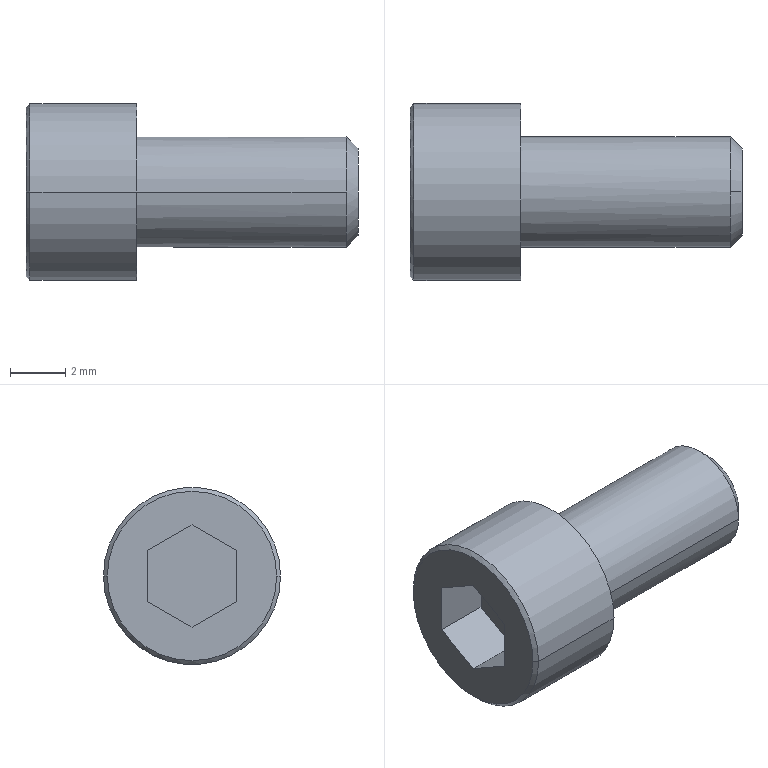Part | NX | features BREP 1 | 1 solid | 18 faces | box 12 x 6.4 x 6.4 mm | volume 210.2 mm3 | plane 10 | cylinder 4 | cone 4 | commonest cylinder face diameters 4 x2 6.4 x2
STEP:
#1=CARTESIAN_POINT('',(4.,2.,0.));
#2=VERTEX_POINT('',#1);
#3=CARTESIAN_POINT('',(4.,-2.,0.));
#4=VERTEX_POINT('',#3);
#5=CARTESIAN_POINT('',(4.,0.,0.));
#6=DIRECTION('',(1.,0.,0.));
#7=DIRECTION('',(0.,1.,0.));
#8=AXIS2_PLACEMENT_3D('',#5,#6,#7);
#9=CIRCLE('',#8,2.);
#10=EDGE_CURVE('',#2,#4,#9,.T.);
#11=ORIENTED_EDGE('',*,*,#10,.T.);
#12=CARTESIAN_POINT('',(11.57,-2.,0.));
#13=VERTEX_POINT('',#12);
#14=CARTESIAN_POINT('',(0.,-2.,0.));
#15=DIRECTION('',(1.,0.,0.));
#16=VECTOR('',#15,1000.);
#17=LINE('',#14,#16);
#18=EDGE_CURVE('',#4,#13,#17,.T.);
#19=ORIENTED_EDGE('',*,*,#18,.T.);
#20=CARTESIAN_POINT('',(11.57,0.,2.));
#21=VERTEX_POINT('',#20);
#22=CARTESIAN_POINT('',(11.57,0.,0.));
#23=DIRECTION('',(-1.,0.,0.));
#24=DIRECTION('',(0.,1.,0.));
#25=AXIS2_PLACEMENT_3D('',#22,#23,#24);
#26=CIRCLE('',#25,2.);
#27=EDGE_CURVE('',#13,#21,#26,.T.);
#28=ORIENTED_EDGE('',*,*,#27,.T.);
#29=CARTESIAN_POINT('',(11.57,2.,0.));
#30=VERTEX_POINT('',#29);
#31=CARTESIAN_POINT('',(11.57,0.,0.));
#32=DIRECTION('',(-1.,0.,0.));
#33=DIRECTION('',(0.,1.,0.));
#34=AXIS2_PLACEMENT_3D('',#31,#32,#33);
#35=CIRCLE('',#34,2.);
#36=EDGE_CURVE('',#21,#30,#35,.T.);
#37=ORIENTED_EDGE('',*,*,#36,.T.);
#38=CARTESIAN_POINT('',(0.,2.,0.));
#39=DIRECTION('',(1.,0.,0.));
#40=VECTOR('',#39,1000.);
#41=LINE('',#38,#40);
#42=EDGE_CURVE('',#2,#30,#41,.T.);
#43=ORIENTED_EDGE('',*,*,#42,.F.);
#44=EDGE_LOOP('',(#11,#19,#28,#37,#43));
#45=FACE_BOUND('',#44,.T.);
#46=CARTESIAN_POINT('',(0.,0.,0.));
#47=DIRECTION('',(1.,0.,0.));
#48=DIRECTION('',(0.,-1.,0.));
#49=AXIS2_PLACEMENT_3D('',#46,#47,#48);
#50=CYLINDRICAL_SURFACE('',#49,2.);
#51=ADVANCED_FACE('',(#45),#50,.T.);
#52=CARTESIAN_POINT('',(12.,0.,1.571));
#53=VERTEX_POINT('',#52);
#54=CARTESIAN_POINT('',(12.,0.,-1.571));
#55=VERTEX_POINT('',#54);
#56=CARTESIAN_POINT('',(12.,0.,0.));
#57=DIRECTION('',(-1.,0.,0.));
#58=DIRECTION('',(0.,0.,1.));
#59=AXIS2_PLACEMENT_3D('',#56,#57,#58);
#60=CIRCLE('',#59,1.571);
#61=EDGE_CURVE('',#53,#55,#60,.T.);
#62=ORIENTED_EDGE('',*,*,#61,.T.);
#63=CARTESIAN_POINT('',(11.57,0.,-2.));
#64=VERTEX_POINT('',#63);
#65=CARTESIAN_POINT('',(11.571,0.,-2.));
#66=DIRECTION('',(-0.7071,0.,-0.7071));
#67=VECTOR('',#66,1000.);
#68=LINE('',#65,#67);
#69=EDGE_CURVE('',#55,#64,#68,.T.);
#70=ORIENTED_EDGE('',*,*,#69,.T.);
#71=CARTESIAN_POINT('',(11.57,0.,0.));
#72=DIRECTION('',(-1.,0.,0.));
#73=DIRECTION('',(0.,1.,0.));
#74=AXIS2_PLACEMENT_3D('',#71,#72,#73);
#75=CIRCLE('',#74,2.);
#76=EDGE_CURVE('',#30,#64,#75,.T.);
#77=ORIENTED_EDGE('',*,*,#76,.F.);
#78=ORIENTED_EDGE('',*,*,#36,.F.);
#79=CARTESIAN_POINT('',(11.571,0.,2.));
#80=DIRECTION('',(-0.7071,0.,0.7071));
#81=VECTOR('',#80,1000.);
#82=LINE('',#79,#81);
#83=EDGE_CURVE('',#53,#21,#82,.T.);
#84=ORIENTED_EDGE('',*,*,#83,.F.);
#85=EDGE_LOOP('',(#62,#70,#77,#78,#84));
#86=FACE_BOUND('',#85,.T.);
#87=CARTESIAN_POINT('',(11.571,0.,0.));
#88=DIRECTION('',(-1.,0.,0.));
#89=DIRECTION('',(0.,0.,-1.));
#90=AXIS2_PLACEMENT_3D('',#87,#88,#89);
#91=CONICAL_SURFACE('',#90,2.,0.7854);
#92=ADVANCED_FACE('',(#86),#91,.T.);
#93=CARTESIAN_POINT('',(0.1414,3.2,0.));
#94=VERTEX_POINT('',#93);
#95=CARTESIAN_POINT('',(0.1414,-3.2,0.));
#96=VERTEX_POINT('',#95);
#97=CARTESIAN_POINT('',(0.1414,0.,0.));
#98=DIRECTION('',(1.,0.,0.));
#99=DIRECTION('',(0.,1.,0.));
#100=AXIS2_PLACEMENT_3D('',#97,#98,#99);
#101=CIRCLE('',#100,3.2);
#102=EDGE_CURVE('',#94,#96,#101,.T.);
#103=ORIENTED_EDGE('',*,*,#102,.T.);
#104=CARTESIAN_POINT('',(4.,-3.2,0.));
#105=VERTEX_POINT('',#104);
#106=CARTESIAN_POINT('',(0.,-3.2,0.));
#107=DIRECTION('',(1.,0.,0.));
#108=VECTOR('',#107,1000.);
#109=LINE('',#106,#108);
#110=EDGE_CURVE('',#96,#105,#109,.T.);
#111=ORIENTED_EDGE('',*,*,#110,.T.);
#112=CARTESIAN_POINT('',(4.,3.2,0.));
#113=VERTEX_POINT('',#112);
#114=CARTESIAN_POINT('',(4.,0.,0.));
#115=DIRECTION('',(-1.,0.,0.));
#116=DIRECTION('',(0.,1.,0.));
#117=AXIS2_PLACEMENT_3D('',#114,#115,#116);
#118=CIRCLE('',#117,3.2);
#119=EDGE_CURVE('',#105,#113,#118,.T.);
#120=ORIENTED_EDGE('',*,*,#119,.T.);
#121=CARTESIAN_POINT('',(0.,3.2,0.));
#122=DIRECTION('',(1.,0.,0.));
#123=VECTOR('',#122,1000.);
#124=LINE('',#121,#123);
#125=EDGE_CURVE('',#94,#113,#124,.T.);
#126=ORIENTED_EDGE('',*,*,#125,.F.);
#127=EDGE_LOOP('',(#103,#111,#120,#126));
#128=FACE_BOUND('',#127,.T.);
#129=CARTESIAN_POINT('',(0.,0.,0.));
#130=DIRECTION('',(1.,0.,0.));
#131=DIRECTION('',(0.,-1.,0.));
#132=AXIS2_PLACEMENT_3D('',#129,#130,#131);
#133=CYLINDRICAL_SURFACE('',#132,3.2);
#134=ADVANCED_FACE('',(#128),#133,.T.);
#135=CARTESIAN_POINT('',(0.,3.059,0.));
#136=VERTEX_POINT('',#135);
#137=CARTESIAN_POINT('',(0.,-3.059,0.));
#138=VERTEX_POINT('',#137);
#139=CARTESIAN_POINT('',(0.,0.,0.));
#140=DIRECTION('',(1.,0.,0.));
#141=DIRECTION('',(0.,1.,0.));
#142=AXIS2_PLACEMENT_3D('',#139,#140,#141);
#143=CIRCLE('',#142,3.059);
#144=EDGE_CURVE('',#136,#138,#143,.T.);
#145=ORIENTED_EDGE('',*,*,#144,.T.);
#146=CARTESIAN_POINT('',(0.1414,-3.2,0.));
#147=DIRECTION('',(0.7071,-0.7071,0.));
#148=VECTOR('',#147,1000.);
#149=LINE('',#146,#148);
#150=EDGE_CURVE('',#138,#96,#149,.T.);
#151=ORIENTED_EDGE('',*,*,#150,.T.);
#152=ORIENTED_EDGE('',*,*,#102,.F.);
#153=CARTESIAN_POINT('',(0.1414,3.2,0.));
#154=DIRECTION('',(0.7071,0.7071,0.));
#155=VECTOR('',#154,1000.);
#156=LINE('',#153,#155);
#157=EDGE_CURVE('',#136,#94,#156,.T.);
#158=ORIENTED_EDGE('',*,*,#157,.F.);
#159=EDGE_LOOP('',(#145,#151,#152,#158));
#160=FACE_BOUND('',#159,.T.);
#161=CARTESIAN_POINT('',(0.1414,0.,0.));
#162=DIRECTION('',(1.,0.,0.));
#163=DIRECTION('',(0.,-1.,0.));
#164=AXIS2_PLACEMENT_3D('',#161,#162,#163);
#165=CONICAL_SURFACE('',#164,3.2,0.7854);
#166=ADVANCED_FACE('',(#160),#165,.T.);
#167=ORIENTED_EDGE('',*,*,#18,.F.);
#168=CARTESIAN_POINT('',(4.,0.,0.));
#169=DIRECTION('',(1.,0.,0.));
#170=DIRECTION('',(0.,1.,0.));
#171=AXIS2_PLACEMENT_3D('',#168,#169,#170);
#172=CIRCLE('',#171,2.);
#173=EDGE_CURVE('',#4,#2,#172,.T.);
#174=ORIENTED_EDGE('',*,*,#173,.T.);
#175=ORIENTED_EDGE('',*,*,#42,.T.);
#176=ORIENTED_EDGE('',*,*,#76,.T.);
#177=CARTESIAN_POINT('',(11.57,0.,0.));
#178=DIRECTION('',(-1.,0.,0.));
#179=DIRECTION('',(0.,1.,0.));
#180=AXIS2_PLACEMENT_3D('',#177,#178,#179);
#181=CIRCLE('',#180,2.);
#182=EDGE_CURVE('',#64,#13,#181,.T.);
#183=ORIENTED_EDGE('',*,*,#182,.T.);
#184=EDGE_LOOP('',(#167,#174,#175,#176,#183));
#185=FACE_BOUND('',#184,.T.);
#186=CARTESIAN_POINT('',(0.,0.,0.));
#187=DIRECTION('',(1.,0.,0.));
#188=DIRECTION('',(0.,-1.,0.));
#189=AXIS2_PLACEMENT_3D('',#186,#187,#188);
#190=CYLINDRICAL_SURFACE('',#189,2.);
#191=ADVANCED_FACE('',(#185),#190,.T.);
#192=ORIENTED_EDGE('',*,*,#69,.F.);
#193=CARTESIAN_POINT('',(12.,0.,0.));
#194=DIRECTION('',(-1.,0.,0.));
#195=DIRECTION('',(0.,0.,1.));
#196=AXIS2_PLACEMENT_3D('',#193,#194,#195);
#197=CIRCLE('',#196,1.571);
#198=EDGE_CURVE('',#55,#53,#197,.T.);
#199=ORIENTED_EDGE('',*,*,#198,.T.);
#200=ORIENTED_EDGE('',*,*,#83,.T.);
#201=ORIENTED_EDGE('',*,*,#27,.F.);
#202=ORIENTED_EDGE('',*,*,#182,.F.);
#203=EDGE_LOOP('',(#192,#199,#200,#201,#202));
#204=FACE_BOUND('',#203,.T.);
#205=CARTESIAN_POINT('',(11.571,0.,0.));
#206=DIRECTION('',(-1.,0.,0.));
#207=DIRECTION('',(0.,0.,-1.));
#208=AXIS2_PLACEMENT_3D('',#205,#206,#207);
#209=CONICAL_SURFACE('',#208,2.,0.7854);
#210=ADVANCED_FACE('',(#204),#209,.T.);
#211=ORIENTED_EDGE('',*,*,#10,.F.);
#212=ORIENTED_EDGE('',*,*,#173,.F.);
#213=EDGE_LOOP('',(#211,#212));
#214=FACE_BOUND('',#213,.T.);
#215=CARTESIAN_POINT('',(4.,0.,0.));
#216=DIRECTION('',(-1.,0.,0.));
#217=DIRECTION('',(0.,1.,0.));
#218=AXIS2_PLACEMENT_3D('',#215,#216,#217);
#219=CIRCLE('',#218,3.2);
#220=EDGE_CURVE('',#113,#105,#219,.T.);
#221=ORIENTED_EDGE('',*,*,#220,.F.);
#222=ORIENTED_EDGE('',*,*,#119,.F.);
#223=EDGE_LOOP('',(#221,#222));
#224=FACE_BOUND('',#223,.T.);
#225=CARTESIAN_POINT('',(4.,-2.,0.));
#226=DIRECTION('',(-1.,0.,0.));
#227=DIRECTION('',(0.,1.,0.));
#228=AXIS2_PLACEMENT_3D('',#225,#226,#227);
#229=PLANE('',#228);
#230=ADVANCED_FACE('',(#214,#224),#229,.F.);
#231=ORIENTED_EDGE('',*,*,#61,.F.);
#232=ORIENTED_EDGE('',*,*,#198,.F.);
#233=EDGE_LOOP('',(#231,#232));
#234=FACE_BOUND('',#233,.T.);
#235=CARTESIAN_POINT('',(12.,0.,0.));
#236=DIRECTION('',(-1.,0.,0.));
#237=DIRECTION('',(0.,1.,0.));
#238=AXIS2_PLACEMENT_3D('',#235,#236,#237);
#239=PLANE('',#238);
#240=ADVANCED_FACE('',(#234),#239,.F.);
#241=ORIENTED_EDGE('',*,*,#110,.F.);
#242=CARTESIAN_POINT('',(0.1414,0.,0.));
#243=DIRECTION('',(1.,0.,0.));
#244=DIRECTION('',(0.,1.,0.));
#245=AXIS2_PLACEMENT_3D('',#242,#243,#244);
#246=CIRCLE('',#245,3.2);
#247=EDGE_CURVE('',#96,#94,#246,.T.);
#248=ORIENTED_EDGE('',*,*,#247,.T.);
#249=ORIENTED_EDGE('',*,*,#125,.T.);
#250=ORIENTED_EDGE('',*,*,#220,.T.);
#251=EDGE_LOOP('',(#241,#248,#249,#250));
#252=FACE_BOUND('',#251,.T.);
#253=CARTESIAN_POINT('',(0.,0.,0.));
#254=DIRECTION('',(1.,0.,0.));
#255=DIRECTION('',(0.,-1.,0.));
#256=AXIS2_PLACEMENT_3D('',#253,#254,#255);
#257=CYLINDRICAL_SURFACE('',#256,3.2);
#258=ADVANCED_FACE('',(#252),#257,.T.);
#259=ORIENTED_EDGE('',*,*,#150,.F.);
#260=CARTESIAN_POINT('',(0.,0.,0.));
#261=DIRECTION('',(1.,0.,0.));
#262=DIRECTION('',(0.,1.,0.));
#263=AXIS2_PLACEMENT_3D('',#260,#261,#262);
#264=CIRCLE('',#263,3.059);
#265=EDGE_CURVE('',#138,#136,#264,.T.);
#266=ORIENTED_EDGE('',*,*,#265,.T.);
#267=ORIENTED_EDGE('',*,*,#157,.T.);
#268=ORIENTED_EDGE('',*,*,#247,.F.);
#269=EDGE_LOOP('',(#259,#266,#267,#268));
#270=FACE_BOUND('',#269,.T.);
#271=CARTESIAN_POINT('',(0.1414,0.,0.));
#272=DIRECTION('',(1.,0.,0.));
#273=DIRECTION('',(0.,-1.,0.));
#274=AXIS2_PLACEMENT_3D('',#271,#272,#273);
#275=CONICAL_SURFACE('',#274,3.2,0.7854);
#276=ADVANCED_FACE('',(#270),#275,.T.);
#277=ORIENTED_EDGE('',*,*,#144,.F.);
#278=ORIENTED_EDGE('',*,*,#265,.F.);
#279=EDGE_LOOP('',(#277,#278));
#280=FACE_BOUND('',#279,.T.);
#281=CARTESIAN_POINT('',(0.,0.,-1.848));
#282=VERTEX_POINT('',#281);
#283=CARTESIAN_POINT('',(0.,-1.6,-0.9238));
#284=VERTEX_POINT('',#283);
#285=CARTESIAN_POINT('',(0.,0.,-1.848));
#286=DIRECTION('',(0.,-0.866,0.5));
#287=VECTOR('',#286,1000.);
#288=LINE('',#285,#287);
#289=EDGE_CURVE('',#282,#284,#288,.T.);
#290=ORIENTED_EDGE('',*,*,#289,.F.);
#291=CARTESIAN_POINT('',(0.,1.6,-0.9238));
#292=VERTEX_POINT('',#291);
#293=CARTESIAN_POINT('',(0.,1.6,-0.9238));
#294=DIRECTION('',(0.,-0.866,-0.5));
#295=VECTOR('',#294,1000.);
#296=LINE('',#293,#295);
#297=EDGE_CURVE('',#292,#282,#296,.T.);
#298=ORIENTED_EDGE('',*,*,#297,.F.);
#299=CARTESIAN_POINT('',(0.,1.6,0.9238));
#300=VERTEX_POINT('',#299);
#301=CARTESIAN_POINT('',(0.,1.6,0.));
#302=DIRECTION('',(0.,0.,-1.));
#303=VECTOR('',#302,1000.);
#304=LINE('',#301,#303);
#305=EDGE_CURVE('',#300,#292,#304,.T.);
#306=ORIENTED_EDGE('',*,*,#305,.F.);
#307=CARTESIAN_POINT('',(0.,0.,1.848));
#308=VERTEX_POINT('',#307);
#309=CARTESIAN_POINT('',(0.,0.,1.848));
#310=DIRECTION('',(0.,0.866,-0.5));
#311=VECTOR('',#310,1000.);
#312=LINE('',#309,#311);
#313=EDGE_CURVE('',#308,#300,#312,.T.);
#314=ORIENTED_EDGE('',*,*,#313,.F.);
#315=CARTESIAN_POINT('',(0.,-1.6,0.9238));
#316=VERTEX_POINT('',#315);
#317=CARTESIAN_POINT('',(0.,-1.6,0.9238));
#318=DIRECTION('',(0.,0.866,0.5));
#319=VECTOR('',#318,1000.);
#320=LINE('',#317,#319);
#321=EDGE_CURVE('',#316,#308,#320,.T.);
#322=ORIENTED_EDGE('',*,*,#321,.F.);
#323=CARTESIAN_POINT('',(0.,-1.6,0.));
#324=DIRECTION('',(0.,0.,1.));
#325=VECTOR('',#324,1000.);
#326=LINE('',#323,#325);
#327=EDGE_CURVE('',#284,#316,#326,.T.);
#328=ORIENTED_EDGE('',*,*,#327,.F.);
#329=EDGE_LOOP('',(#290,#298,#306,#314,#322,#328));
#330=FACE_BOUND('',#329,.T.);
#331=CARTESIAN_POINT('',(0.,-3.059,0.));
#332=DIRECTION('',(1.,0.,0.));
#333=DIRECTION('',(0.,-1.,0.));
#334=AXIS2_PLACEMENT_3D('',#331,#332,#333);
#335=PLANE('',#334);
#336=ADVANCED_FACE('',(#280,#330),#335,.F.);
#337=ORIENTED_EDGE('',*,*,#327,.T.);
#338=CARTESIAN_POINT('',(2.,-1.6,0.9238));
#339=VERTEX_POINT('',#338);
#340=CARTESIAN_POINT('',(2.,-1.6,0.9238));
#341=DIRECTION('',(-1.,0.,0.));
#342=VECTOR('',#341,1000.);
#343=LINE('',#340,#342);
#344=EDGE_CURVE('',#339,#316,#343,.T.);
#345=ORIENTED_EDGE('',*,*,#344,.F.);
#346=CARTESIAN_POINT('',(2.,-1.6,-0.9238));
#347=VERTEX_POINT('',#346);
#348=CARTESIAN_POINT('',(2.,-1.6,-0.9238));
#349=DIRECTION('',(0.,0.,1.));
#350=VECTOR('',#349,1000.);
#351=LINE('',#348,#350);
#352=EDGE_CURVE('',#347,#339,#351,.T.);
#353=ORIENTED_EDGE('',*,*,#352,.F.);
#354=CARTESIAN_POINT('',(2.,-1.6,-0.9238));
#355=DIRECTION('',(1.,0.,0.));
#356=VECTOR('',#355,1000.);
#357=LINE('',#354,#356);
#358=EDGE_CURVE('',#284,#347,#357,.T.);
#359=ORIENTED_EDGE('',*,*,#358,.F.);
#360=EDGE_LOOP('',(#337,#345,#353,#359));
#361=FACE_BOUND('',#360,.T.);
#362=CARTESIAN_POINT('',(2.,-1.6,-0.9238));
#363=DIRECTION('',(0.,-1.,0.));
#364=DIRECTION('',(0.,0.,1.));
#365=AXIS2_PLACEMENT_3D('',#362,#363,#364);
#366=PLANE('',#365);
#367=ADVANCED_FACE('',(#361),#366,.F.);
#368=ORIENTED_EDGE('',*,*,#358,.T.);
#369=CARTESIAN_POINT('',(2.,0.,-1.848));
#370=VERTEX_POINT('',#369);
#371=CARTESIAN_POINT('',(2.,0.,-1.848));
#372=DIRECTION('',(0.,-0.866,0.5));
#373=VECTOR('',#372,1000.);
#374=LINE('',#371,#373);
#375=EDGE_CURVE('',#370,#347,#374,.T.);
#376=ORIENTED_EDGE('',*,*,#375,.F.);
#377=CARTESIAN_POINT('',(2.,0.,-1.848));
#378=DIRECTION('',(1.,0.,0.));
#379=VECTOR('',#378,1000.);
#380=LINE('',#377,#379);
#381=EDGE_CURVE('',#282,#370,#380,.T.);
#382=ORIENTED_EDGE('',*,*,#381,.F.);
#383=ORIENTED_EDGE('',*,*,#289,.T.);
#384=EDGE_LOOP('',(#368,#376,#382,#383));
#385=FACE_BOUND('',#384,.T.);
#386=CARTESIAN_POINT('',(2.,0.,-1.848));
#387=DIRECTION('',(0.,-0.5,-0.866));
#388=DIRECTION('',(0.,-0.866,0.5));
#389=AXIS2_PLACEMENT_3D('',#386,#387,#388);
#390=PLANE('',#389);
#391=ADVANCED_FACE('',(#385),#390,.F.);
#392=ORIENTED_EDGE('',*,*,#381,.T.);
#393=CARTESIAN_POINT('',(2.,1.6,-0.9238));
#394=VERTEX_POINT('',#393);
#395=CARTESIAN_POINT('',(2.,1.6,-0.9238));
#396=DIRECTION('',(0.,-0.866,-0.5));
#397=VECTOR('',#396,1000.);
#398=LINE('',#395,#397);
#399=EDGE_CURVE('',#394,#370,#398,.T.);
#400=ORIENTED_EDGE('',*,*,#399,.F.);
#401=CARTESIAN_POINT('',(2.,1.6,-0.9238));
#402=DIRECTION('',(1.,0.,0.));
#403=VECTOR('',#402,1000.);
#404=LINE('',#401,#403);
#405=EDGE_CURVE('',#292,#394,#404,.T.);
#406=ORIENTED_EDGE('',*,*,#405,.F.);
#407=ORIENTED_EDGE('',*,*,#297,.T.);
#408=EDGE_LOOP('',(#392,#400,#406,#407));
#409=FACE_BOUND('',#408,.T.);
#410=CARTESIAN_POINT('',(2.,1.6,-0.9238));
#411=DIRECTION('',(0.,0.5,-0.866));
#412=DIRECTION('',(0.,-0.866,-0.5));
#413=AXIS2_PLACEMENT_3D('',#410,#411,#412);
#414=PLANE('',#413);
#415=ADVANCED_FACE('',(#409),#414,.F.);
#416=ORIENTED_EDGE('',*,*,#405,.T.);
#417=CARTESIAN_POINT('',(2.,1.6,0.9238));
#418=VERTEX_POINT('',#417);
#419=CARTESIAN_POINT('',(2.,1.6,0.9238));
#420=DIRECTION('',(0.,0.,-1.));
#421=VECTOR('',#420,1000.);
#422=LINE('',#419,#421);
#423=EDGE_CURVE('',#418,#394,#422,.T.);
#424=ORIENTED_EDGE('',*,*,#423,.F.);
#425=CARTESIAN_POINT('',(2.,1.6,0.9238));
#426=DIRECTION('',(1.,0.,0.));
#427=VECTOR('',#426,1000.);
#428=LINE('',#425,#427);
#429=EDGE_CURVE('',#300,#418,#428,.T.);
#430=ORIENTED_EDGE('',*,*,#429,.F.);
#431=ORIENTED_EDGE('',*,*,#305,.T.);
#432=EDGE_LOOP('',(#416,#424,#430,#431));
#433=FACE_BOUND('',#432,.T.);
#434=CARTESIAN_POINT('',(2.,1.6,0.9238));
#435=DIRECTION('',(0.,1.,0.));
#436=DIRECTION('',(0.,0.,-1.));
#437=AXIS2_PLACEMENT_3D('',#434,#435,#436);
#438=PLANE('',#437);
#439=ADVANCED_FACE('',(#433),#438,.F.);
#440=ORIENTED_EDGE('',*,*,#429,.T.);
#441=CARTESIAN_POINT('',(2.,0.,1.848));
#442=VERTEX_POINT('',#441);
#443=CARTESIAN_POINT('',(2.,0.,1.848));
#444=DIRECTION('',(0.,0.866,-0.5));
#445=VECTOR('',#444,1000.);
#446=LINE('',#443,#445);
#447=EDGE_CURVE('',#442,#418,#446,.T.);
#448=ORIENTED_EDGE('',*,*,#447,.F.);
#449=CARTESIAN_POINT('',(2.,0.,1.848));
#450=DIRECTION('',(1.,0.,0.));
#451=VECTOR('',#450,1000.);
#452=LINE('',#449,#451);
#453=EDGE_CURVE('',#308,#442,#452,.T.);
#454=ORIENTED_EDGE('',*,*,#453,.F.);
#455=ORIENTED_EDGE('',*,*,#313,.T.);
#456=EDGE_LOOP('',(#440,#448,#454,#455));
#457=FACE_BOUND('',#456,.T.);
#458=CARTESIAN_POINT('',(2.,0.,1.848));
#459=DIRECTION('',(0.,0.5,0.866));
#460=DIRECTION('',(0.,0.866,-0.5));
#461=AXIS2_PLACEMENT_3D('',#458,#459,#460);
#462=PLANE('',#461);
#463=ADVANCED_FACE('',(#457),#462,.F.);
#464=ORIENTED_EDGE('',*,*,#453,.T.);
#465=CARTESIAN_POINT('',(2.,-1.6,0.9238));
#466=DIRECTION('',(0.,0.866,0.5));
#467=VECTOR('',#466,1000.);
#468=LINE('',#465,#467);
#469=EDGE_CURVE('',#339,#442,#468,.T.);
#470=ORIENTED_EDGE('',*,*,#469,.F.);
#471=ORIENTED_EDGE('',*,*,#344,.T.);
#472=ORIENTED_EDGE('',*,*,#321,.T.);
#473=EDGE_LOOP('',(#464,#470,#471,#472));
#474=FACE_BOUND('',#473,.T.);
#475=CARTESIAN_POINT('',(2.,-1.6,0.9238));
#476=DIRECTION('',(0.,-0.5,0.866));
#477=DIRECTION('',(0.,0.866,0.5));
#478=AXIS2_PLACEMENT_3D('',#475,#476,#477);
#479=PLANE('',#478);
#480=ADVANCED_FACE('',(#474),#479,.F.);
#481=ORIENTED_EDGE('',*,*,#469,.T.);
#482=ORIENTED_EDGE('',*,*,#447,.T.);
#483=ORIENTED_EDGE('',*,*,#423,.T.);
#484=ORIENTED_EDGE('',*,*,#399,.T.);
#485=ORIENTED_EDGE('',*,*,#375,.T.);
#486=ORIENTED_EDGE('',*,*,#352,.T.);
#487=EDGE_LOOP('',(#481,#482,#483,#484,#485,#486));
#488=FACE_BOUND('',#487,.T.);
#489=CARTESIAN_POINT('',(2.,0.,0.));
#490=DIRECTION('',(-1.,0.,0.));
#491=DIRECTION('',(0.,0.,-1.));
#492=AXIS2_PLACEMENT_3D('',#489,#490,#491);
#493=PLANE('',#492);
#494=ADVANCED_FACE('',(#488),#493,.T.);
#495=CLOSED_SHELL('',(#51,#92,#134,#166,#191,#210,#230,#240,#258,#276,#336,#367,#391,#415,#439,#463,#480,#494));
#496=MANIFOLD_SOLID_BREP('',#495);
#497=(LENGTH_UNIT()NAMED_UNIT(*)SI_UNIT(.MILLI.,.METRE.));
#498=UNCERTAINTY_MEASURE_WITH_UNIT(LENGTH_MEASURE(0.00001),#497,'','');
#499=(NAMED_UNIT(*)PLANE_ANGLE_UNIT()SI_UNIT($,.RADIAN.));
#500=(NAMED_UNIT(*)SI_UNIT($,.STERADIAN.)SOLID_ANGLE_UNIT());
#501=(GEOMETRIC_REPRESENTATION_CONTEXT(3)GLOBAL_UNCERTAINTY_ASSIGNED_CONTEXT((#498))GLOBAL_UNIT_ASSIGNED_CONTEXT((#497,#499,#500))REPRESENTATION_CONTEXT('',''));
#502=ADVANCED_BREP_SHAPE_REPRESENTATION('',(#496),#501);